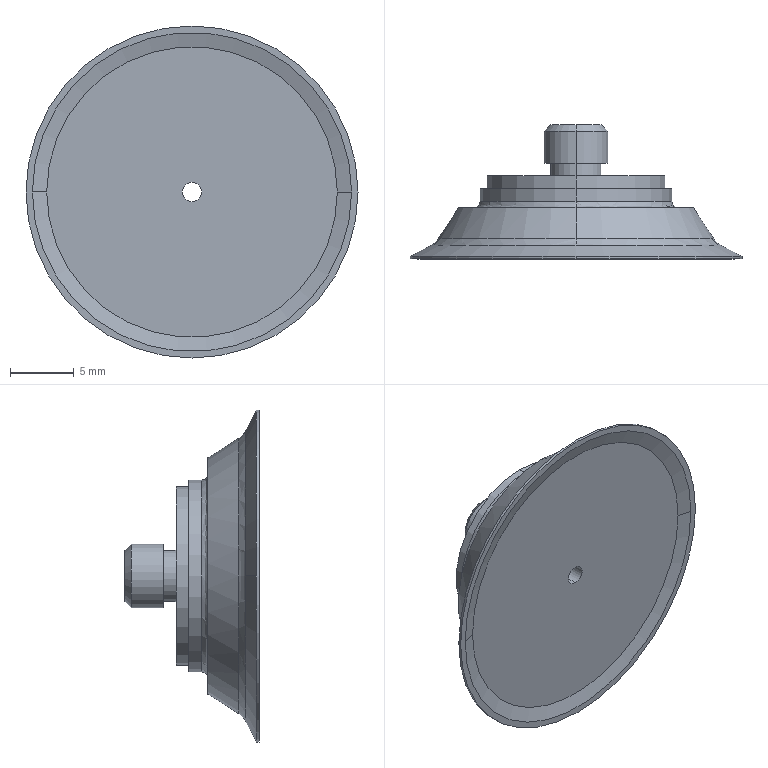Part | SolidWorks | features BaseBody 2 | 2 solids | 58 faces | box 26 x 10.5 x 26 mm | volume 1762 mm3 | plane 24 | cylinder 22 | cone 8 | spline 4 | commonest cylinder face diameters 6.1 x4 1.5 x2 2.5 x2 4 x2 5 x2 9.4 x2